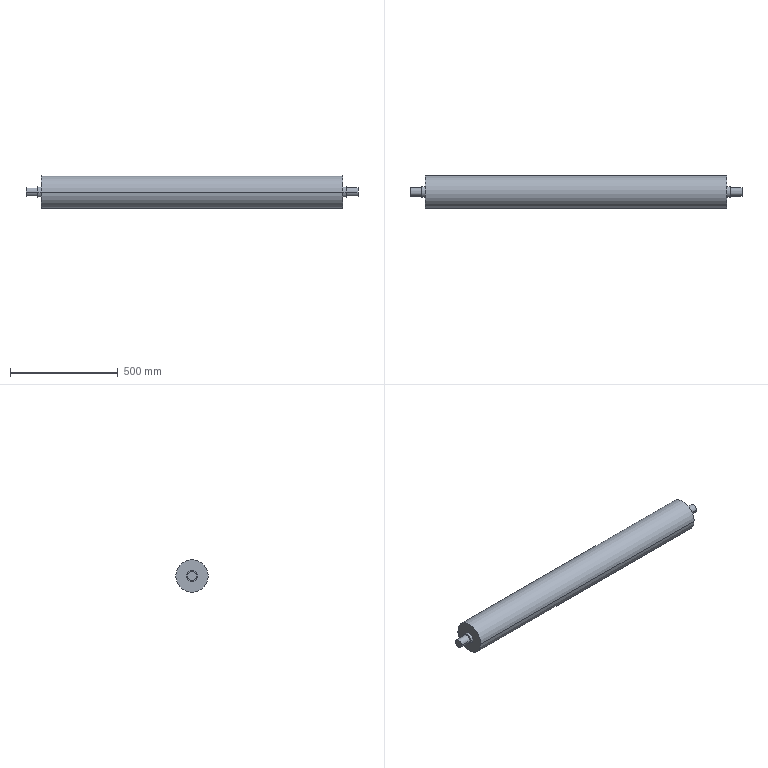Part | SolidWorks | features BaseBody 1 | 1 solid | 16 faces | box 1540 x 150 x 150 mm | volume 24937177 mm3 | cylinder 10 | plane 6 | commonest cylinder face diameters 40 x4 50 x4 150 x2
STEP:
#1=CARTESIAN_POINT('',(-715.,-20.,0.));
#2=VERTEX_POINT('',#1);
#3=CARTESIAN_POINT('',(-715.,20.,0.));
#4=VERTEX_POINT('',#3);
#5=CARTESIAN_POINT('',(-715.,0.,0.));
#6=DIRECTION('',(-1.,0.,0.));
#7=DIRECTION('',(0.,1.,0.));
#8=AXIS2_PLACEMENT_3D('',#5,#6,#7);
#9=CIRCLE('',#8,20.);
#10=EDGE_CURVE('',#2,#4,#9,.T.);
#11=ORIENTED_EDGE('',*,*,#10,.T.);
#12=CARTESIAN_POINT('',(-770.,20.,0.));
#13=VERTEX_POINT('',#12);
#14=CARTESIAN_POINT('',(-820.,20.,0.));
#15=DIRECTION('',(-1.,0.,0.));
#16=VECTOR('',#15,1000.);
#17=LINE('',#14,#16);
#18=EDGE_CURVE('',#4,#13,#17,.T.);
#19=ORIENTED_EDGE('',*,*,#18,.T.);
#20=CARTESIAN_POINT('',(-770.,-20.,0.));
#21=VERTEX_POINT('',#20);
#22=CARTESIAN_POINT('',(-770.,0.,0.));
#23=DIRECTION('',(-1.,0.,0.));
#24=DIRECTION('',(0.,-1.,0.));
#25=AXIS2_PLACEMENT_3D('',#22,#23,#24);
#26=CIRCLE('',#25,20.);
#27=EDGE_CURVE('',#21,#13,#26,.T.);
#28=ORIENTED_EDGE('',*,*,#27,.F.);
#29=CARTESIAN_POINT('',(-820.,-20.,0.));
#30=DIRECTION('',(-1.,0.,0.));
#31=VECTOR('',#30,1000.);
#32=LINE('',#29,#31);
#33=EDGE_CURVE('',#2,#21,#32,.T.);
#34=ORIENTED_EDGE('',*,*,#33,.F.);
#35=EDGE_LOOP('',(#11,#19,#28,#34));
#36=FACE_OUTER_BOUND('',#35,.T.);
#37=CARTESIAN_POINT('',(-820.,0.,0.));
#38=DIRECTION('',(-1.,0.,0.));
#39=DIRECTION('',(0.,-1.,0.));
#40=AXIS2_PLACEMENT_3D('',#37,#38,#39);
#41=CYLINDRICAL_SURFACE('',#40,20.);
#42=ADVANCED_FACE('',(#36),#41,.T.);
#43=CARTESIAN_POINT('',(-700.,-25.,0.));
#44=VERTEX_POINT('',#43);
#45=CARTESIAN_POINT('',(-700.,25.,0.));
#46=VERTEX_POINT('',#45);
#47=CARTESIAN_POINT('',(-700.,0.,0.));
#48=DIRECTION('',(-1.,0.,0.));
#49=DIRECTION('',(0.,1.,0.));
#50=AXIS2_PLACEMENT_3D('',#47,#48,#49);
#51=CIRCLE('',#50,25.);
#52=EDGE_CURVE('',#44,#46,#51,.T.);
#53=ORIENTED_EDGE('',*,*,#52,.T.);
#54=CARTESIAN_POINT('',(-715.,25.,0.));
#55=VERTEX_POINT('',#54);
#56=CARTESIAN_POINT('',(-820.,25.,0.));
#57=DIRECTION('',(-1.,0.,0.));
#58=VECTOR('',#57,1000.);
#59=LINE('',#56,#58);
#60=EDGE_CURVE('',#46,#55,#59,.T.);
#61=ORIENTED_EDGE('',*,*,#60,.T.);
#62=CARTESIAN_POINT('',(-715.,-25.,0.));
#63=VERTEX_POINT('',#62);
#64=CARTESIAN_POINT('',(-715.,0.,0.));
#65=DIRECTION('',(-1.,0.,0.));
#66=DIRECTION('',(0.,-1.,0.));
#67=AXIS2_PLACEMENT_3D('',#64,#65,#66);
#68=CIRCLE('',#67,25.);
#69=EDGE_CURVE('',#63,#55,#68,.T.);
#70=ORIENTED_EDGE('',*,*,#69,.F.);
#71=CARTESIAN_POINT('',(-820.,-25.,0.));
#72=DIRECTION('',(-1.,0.,0.));
#73=VECTOR('',#72,1000.);
#74=LINE('',#71,#73);
#75=EDGE_CURVE('',#44,#63,#74,.T.);
#76=ORIENTED_EDGE('',*,*,#75,.F.);
#77=EDGE_LOOP('',(#53,#61,#70,#76));
#78=FACE_OUTER_BOUND('',#77,.T.);
#79=CARTESIAN_POINT('',(-820.,0.,0.));
#80=DIRECTION('',(-1.,0.,0.));
#81=DIRECTION('',(0.,-1.,0.));
#82=AXIS2_PLACEMENT_3D('',#79,#80,#81);
#83=CYLINDRICAL_SURFACE('',#82,25.);
#84=ADVANCED_FACE('',(#78),#83,.T.);
#85=CARTESIAN_POINT('',(770.,-20.,0.));
#86=VERTEX_POINT('',#85);
#87=CARTESIAN_POINT('',(770.,20.,0.));
#88=VERTEX_POINT('',#87);
#89=CARTESIAN_POINT('',(770.,0.,0.));
#90=DIRECTION('',(-1.,0.,0.));
#91=DIRECTION('',(0.,-1.,0.));
#92=AXIS2_PLACEMENT_3D('',#89,#90,#91);
#93=CIRCLE('',#92,20.);
#94=EDGE_CURVE('',#86,#88,#93,.T.);
#95=ORIENTED_EDGE('',*,*,#94,.T.);
#96=CARTESIAN_POINT('',(715.,20.,0.));
#97=VERTEX_POINT('',#96);
#98=CARTESIAN_POINT('',(-820.,20.,0.));
#99=DIRECTION('',(-1.,0.,0.));
#100=VECTOR('',#99,1000.);
#101=LINE('',#98,#100);
#102=EDGE_CURVE('',#88,#97,#101,.T.);
#103=ORIENTED_EDGE('',*,*,#102,.T.);
#104=CARTESIAN_POINT('',(715.,-20.,0.));
#105=VERTEX_POINT('',#104);
#106=CARTESIAN_POINT('',(715.,0.,0.));
#107=DIRECTION('',(1.,0.,0.));
#108=DIRECTION('',(0.,-1.,0.));
#109=AXIS2_PLACEMENT_3D('',#106,#107,#108);
#110=CIRCLE('',#109,20.);
#111=EDGE_CURVE('',#97,#105,#110,.T.);
#112=ORIENTED_EDGE('',*,*,#111,.T.);
#113=CARTESIAN_POINT('',(-820.,-20.,0.));
#114=DIRECTION('',(-1.,0.,0.));
#115=VECTOR('',#114,1000.);
#116=LINE('',#113,#115);
#117=EDGE_CURVE('',#86,#105,#116,.T.);
#118=ORIENTED_EDGE('',*,*,#117,.F.);
#119=EDGE_LOOP('',(#95,#103,#112,#118));
#120=FACE_OUTER_BOUND('',#119,.T.);
#121=CARTESIAN_POINT('',(-820.,0.,0.));
#122=DIRECTION('',(-1.,0.,0.));
#123=DIRECTION('',(0.,-1.,0.));
#124=AXIS2_PLACEMENT_3D('',#121,#122,#123);
#125=CYLINDRICAL_SURFACE('',#124,20.);
#126=ADVANCED_FACE('',(#120),#125,.T.);
#127=CARTESIAN_POINT('',(715.,-25.,0.));
#128=VERTEX_POINT('',#127);
#129=CARTESIAN_POINT('',(715.,25.,0.));
#130=VERTEX_POINT('',#129);
#131=CARTESIAN_POINT('',(715.,0.,0.));
#132=DIRECTION('',(-1.,0.,0.));
#133=DIRECTION('',(0.,-1.,0.));
#134=AXIS2_PLACEMENT_3D('',#131,#132,#133);
#135=CIRCLE('',#134,25.);
#136=EDGE_CURVE('',#128,#130,#135,.T.);
#137=ORIENTED_EDGE('',*,*,#136,.T.);
#138=CARTESIAN_POINT('',(700.,25.,0.));
#139=VERTEX_POINT('',#138);
#140=CARTESIAN_POINT('',(-820.,25.,0.));
#141=DIRECTION('',(-1.,0.,0.));
#142=VECTOR('',#141,1000.);
#143=LINE('',#140,#142);
#144=EDGE_CURVE('',#130,#139,#143,.T.);
#145=ORIENTED_EDGE('',*,*,#144,.T.);
#146=CARTESIAN_POINT('',(700.,-25.,0.));
#147=VERTEX_POINT('',#146);
#148=CARTESIAN_POINT('',(700.,0.,0.));
#149=DIRECTION('',(1.,0.,0.));
#150=DIRECTION('',(0.,-1.,0.));
#151=AXIS2_PLACEMENT_3D('',#148,#149,#150);
#152=CIRCLE('',#151,25.);
#153=EDGE_CURVE('',#139,#147,#152,.T.);
#154=ORIENTED_EDGE('',*,*,#153,.T.);
#155=CARTESIAN_POINT('',(-820.,-25.,0.));
#156=DIRECTION('',(-1.,0.,0.));
#157=VECTOR('',#156,1000.);
#158=LINE('',#155,#157);
#159=EDGE_CURVE('',#128,#147,#158,.T.);
#160=ORIENTED_EDGE('',*,*,#159,.F.);
#161=EDGE_LOOP('',(#137,#145,#154,#160));
#162=FACE_OUTER_BOUND('',#161,.T.);
#163=CARTESIAN_POINT('',(-820.,0.,0.));
#164=DIRECTION('',(-1.,0.,0.));
#165=DIRECTION('',(0.,-1.,0.));
#166=AXIS2_PLACEMENT_3D('',#163,#164,#165);
#167=CYLINDRICAL_SURFACE('',#166,25.);
#168=ADVANCED_FACE('',(#162),#167,.T.);
#169=CARTESIAN_POINT('',(700.,-75.,0.));
#170=VERTEX_POINT('',#169);
#171=CARTESIAN_POINT('',(700.,75.,0.));
#172=VERTEX_POINT('',#171);
#173=CARTESIAN_POINT('',(700.,0.,0.));
#174=DIRECTION('',(-1.,0.,0.));
#175=DIRECTION('',(0.,-1.,0.));
#176=AXIS2_PLACEMENT_3D('',#173,#174,#175);
#177=CIRCLE('',#176,75.);
#178=EDGE_CURVE('',#170,#172,#177,.T.);
#179=ORIENTED_EDGE('',*,*,#178,.T.);
#180=CARTESIAN_POINT('',(-700.,75.,0.));
#181=VERTEX_POINT('',#180);
#182=CARTESIAN_POINT('',(-820.,75.,0.));
#183=DIRECTION('',(-1.,0.,0.));
#184=VECTOR('',#183,1000.);
#185=LINE('',#182,#184);
#186=EDGE_CURVE('',#172,#181,#185,.T.);
#187=ORIENTED_EDGE('',*,*,#186,.T.);
#188=CARTESIAN_POINT('',(-700.,-75.,0.));
#189=VERTEX_POINT('',#188);
#190=CARTESIAN_POINT('',(-700.,0.,0.));
#191=DIRECTION('',(-1.,0.,0.));
#192=DIRECTION('',(0.,-1.,0.));
#193=AXIS2_PLACEMENT_3D('',#190,#191,#192);
#194=CIRCLE('',#193,75.);
#195=EDGE_CURVE('',#189,#181,#194,.T.);
#196=ORIENTED_EDGE('',*,*,#195,.F.);
#197=CARTESIAN_POINT('',(-820.,-75.,0.));
#198=DIRECTION('',(-1.,0.,0.));
#199=VECTOR('',#198,1000.);
#200=LINE('',#197,#199);
#201=EDGE_CURVE('',#170,#189,#200,.T.);
#202=ORIENTED_EDGE('',*,*,#201,.F.);
#203=EDGE_LOOP('',(#179,#187,#196,#202));
#204=FACE_OUTER_BOUND('',#203,.T.);
#205=CARTESIAN_POINT('',(-820.,0.,0.));
#206=DIRECTION('',(-1.,0.,0.));
#207=DIRECTION('',(0.,-1.,0.));
#208=AXIS2_PLACEMENT_3D('',#205,#206,#207);
#209=CYLINDRICAL_SURFACE('',#208,75.);
#210=ADVANCED_FACE('',(#204),#209,.T.);
#211=ORIENTED_EDGE('',*,*,#27,.T.);
#212=CARTESIAN_POINT('',(-770.,0.,0.));
#213=DIRECTION('',(-1.,0.,0.));
#214=DIRECTION('',(0.,-1.,0.));
#215=AXIS2_PLACEMENT_3D('',#212,#213,#214);
#216=CIRCLE('',#215,20.);
#217=EDGE_CURVE('',#13,#21,#216,.T.);
#218=ORIENTED_EDGE('',*,*,#217,.T.);
#219=EDGE_LOOP('',(#211,#218));
#220=FACE_OUTER_BOUND('',#219,.T.);
#221=CARTESIAN_POINT('',(-770.,17.5,0.));
#222=DIRECTION('',(1.,0.,0.));
#223=DIRECTION('',(0.,-1.,0.));
#224=AXIS2_PLACEMENT_3D('',#221,#222,#223);
#225=PLANE('',#224);
#226=ADVANCED_FACE('',(#220),#225,.F.);
#227=ORIENTED_EDGE('',*,*,#10,.F.);
#228=CARTESIAN_POINT('',(-715.,0.,0.));
#229=DIRECTION('',(-1.,0.,0.));
#230=DIRECTION('',(0.,1.,0.));
#231=AXIS2_PLACEMENT_3D('',#228,#229,#230);
#232=CIRCLE('',#231,20.);
#233=EDGE_CURVE('',#4,#2,#232,.T.);
#234=ORIENTED_EDGE('',*,*,#233,.F.);
#235=EDGE_LOOP('',(#227,#234));
#236=FACE_BOUND('',#235,.T.);
#237=ORIENTED_EDGE('',*,*,#69,.T.);
#238=CARTESIAN_POINT('',(-715.,0.,0.));
#239=DIRECTION('',(-1.,0.,0.));
#240=DIRECTION('',(0.,-1.,0.));
#241=AXIS2_PLACEMENT_3D('',#238,#239,#240);
#242=CIRCLE('',#241,25.);
#243=EDGE_CURVE('',#55,#63,#242,.T.);
#244=ORIENTED_EDGE('',*,*,#243,.T.);
#245=EDGE_LOOP('',(#237,#244));
#246=FACE_OUTER_BOUND('',#245,.T.);
#247=CARTESIAN_POINT('',(-715.,20.,0.));
#248=DIRECTION('',(1.,0.,0.));
#249=DIRECTION('',(0.,-1.,0.));
#250=AXIS2_PLACEMENT_3D('',#247,#248,#249);
#251=PLANE('',#250);
#252=ADVANCED_FACE('',(#236,#246),#251,.F.);
#253=ORIENTED_EDGE('',*,*,#94,.F.);
#254=CARTESIAN_POINT('',(770.,0.,0.));
#255=DIRECTION('',(-1.,0.,0.));
#256=DIRECTION('',(0.,-1.,0.));
#257=AXIS2_PLACEMENT_3D('',#254,#255,#256);
#258=CIRCLE('',#257,20.);
#259=EDGE_CURVE('',#88,#86,#258,.T.);
#260=ORIENTED_EDGE('',*,*,#259,.F.);
#261=EDGE_LOOP('',(#253,#260));
#262=FACE_OUTER_BOUND('',#261,.T.);
#263=CARTESIAN_POINT('',(770.,17.5,0.));
#264=DIRECTION('',(-1.,0.,0.));
#265=DIRECTION('',(0.,0.,1.));
#266=AXIS2_PLACEMENT_3D('',#263,#264,#265);
#267=PLANE('',#266);
#268=ADVANCED_FACE('',(#262),#267,.F.);
#269=CARTESIAN_POINT('',(715.,0.,0.));
#270=DIRECTION('',(1.,0.,0.));
#271=DIRECTION('',(0.,-1.,0.));
#272=AXIS2_PLACEMENT_3D('',#269,#270,#271);
#273=CIRCLE('',#272,20.);
#274=EDGE_CURVE('',#105,#97,#273,.T.);
#275=ORIENTED_EDGE('',*,*,#274,.F.);
#276=ORIENTED_EDGE('',*,*,#111,.F.);
#277=EDGE_LOOP('',(#275,#276));
#278=FACE_BOUND('',#277,.T.);
#279=ORIENTED_EDGE('',*,*,#136,.F.);
#280=CARTESIAN_POINT('',(715.,0.,0.));
#281=DIRECTION('',(-1.,0.,0.));
#282=DIRECTION('',(0.,-1.,0.));
#283=AXIS2_PLACEMENT_3D('',#280,#281,#282);
#284=CIRCLE('',#283,25.);
#285=EDGE_CURVE('',#130,#128,#284,.T.);
#286=ORIENTED_EDGE('',*,*,#285,.F.);
#287=EDGE_LOOP('',(#279,#286));
#288=FACE_OUTER_BOUND('',#287,.T.);
#289=CARTESIAN_POINT('',(715.,20.,0.));
#290=DIRECTION('',(-1.,0.,0.));
#291=DIRECTION('',(0.,0.,1.));
#292=AXIS2_PLACEMENT_3D('',#289,#290,#291);
#293=PLANE('',#292);
#294=ADVANCED_FACE('',(#278,#288),#293,.F.);
#295=CARTESIAN_POINT('',(700.,0.,0.));
#296=DIRECTION('',(1.,0.,0.));
#297=DIRECTION('',(0.,-1.,0.));
#298=AXIS2_PLACEMENT_3D('',#295,#296,#297);
#299=CIRCLE('',#298,25.);
#300=EDGE_CURVE('',#147,#139,#299,.T.);
#301=ORIENTED_EDGE('',*,*,#300,.F.);
#302=ORIENTED_EDGE('',*,*,#153,.F.);
#303=EDGE_LOOP('',(#301,#302));
#304=FACE_BOUND('',#303,.T.);
#305=ORIENTED_EDGE('',*,*,#178,.F.);
#306=CARTESIAN_POINT('',(700.,0.,0.));
#307=DIRECTION('',(-1.,0.,0.));
#308=DIRECTION('',(0.,-1.,0.));
#309=AXIS2_PLACEMENT_3D('',#306,#307,#308);
#310=CIRCLE('',#309,75.);
#311=EDGE_CURVE('',#172,#170,#310,.T.);
#312=ORIENTED_EDGE('',*,*,#311,.F.);
#313=EDGE_LOOP('',(#305,#312));
#314=FACE_OUTER_BOUND('',#313,.T.);
#315=CARTESIAN_POINT('',(700.,75.,0.));
#316=DIRECTION('',(-1.,0.,0.));
#317=DIRECTION('',(0.,0.,1.));
#318=AXIS2_PLACEMENT_3D('',#315,#316,#317);
#319=PLANE('',#318);
#320=ADVANCED_FACE('',(#304,#314),#319,.F.);
#321=ORIENTED_EDGE('',*,*,#52,.F.);
#322=CARTESIAN_POINT('',(-700.,0.,0.));
#323=DIRECTION('',(-1.,0.,0.));
#324=DIRECTION('',(0.,1.,0.));
#325=AXIS2_PLACEMENT_3D('',#322,#323,#324);
#326=CIRCLE('',#325,25.);
#327=EDGE_CURVE('',#46,#44,#326,.T.);
#328=ORIENTED_EDGE('',*,*,#327,.F.);
#329=EDGE_LOOP('',(#321,#328));
#330=FACE_BOUND('',#329,.T.);
#331=ORIENTED_EDGE('',*,*,#195,.T.);
#332=CARTESIAN_POINT('',(-700.,0.,0.));
#333=DIRECTION('',(-1.,0.,0.));
#334=DIRECTION('',(0.,-1.,0.));
#335=AXIS2_PLACEMENT_3D('',#332,#333,#334);
#336=CIRCLE('',#335,75.);
#337=EDGE_CURVE('',#181,#189,#336,.T.);
#338=ORIENTED_EDGE('',*,*,#337,.T.);
#339=EDGE_LOOP('',(#331,#338));
#340=FACE_OUTER_BOUND('',#339,.T.);
#341=CARTESIAN_POINT('',(-700.,75.,0.));
#342=DIRECTION('',(1.,0.,0.));
#343=DIRECTION('',(0.,-1.,0.));
#344=AXIS2_PLACEMENT_3D('',#341,#342,#343);
#345=PLANE('',#344);
#346=ADVANCED_FACE('',(#330,#340),#345,.F.);
#347=ORIENTED_EDGE('',*,*,#186,.F.);
#348=ORIENTED_EDGE('',*,*,#311,.T.);
#349=ORIENTED_EDGE('',*,*,#201,.T.);
#350=ORIENTED_EDGE('',*,*,#337,.F.);
#351=EDGE_LOOP('',(#347,#348,#349,#350));
#352=FACE_OUTER_BOUND('',#351,.T.);
#353=CARTESIAN_POINT('',(-820.,0.,0.));
#354=DIRECTION('',(-1.,0.,0.));
#355=DIRECTION('',(0.,-1.,0.));
#356=AXIS2_PLACEMENT_3D('',#353,#354,#355);
#357=CYLINDRICAL_SURFACE('',#356,75.);
#358=ADVANCED_FACE('',(#352),#357,.T.);
#359=ORIENTED_EDGE('',*,*,#144,.F.);
#360=ORIENTED_EDGE('',*,*,#285,.T.);
#361=ORIENTED_EDGE('',*,*,#159,.T.);
#362=ORIENTED_EDGE('',*,*,#300,.T.);
#363=EDGE_LOOP('',(#359,#360,#361,#362));
#364=FACE_OUTER_BOUND('',#363,.T.);
#365=CARTESIAN_POINT('',(-820.,0.,0.));
#366=DIRECTION('',(-1.,0.,0.));
#367=DIRECTION('',(0.,-1.,0.));
#368=AXIS2_PLACEMENT_3D('',#365,#366,#367);
#369=CYLINDRICAL_SURFACE('',#368,25.);
#370=ADVANCED_FACE('',(#364),#369,.T.);
#371=ORIENTED_EDGE('',*,*,#102,.F.);
#372=ORIENTED_EDGE('',*,*,#259,.T.);
#373=ORIENTED_EDGE('',*,*,#117,.T.);
#374=ORIENTED_EDGE('',*,*,#274,.T.);
#375=EDGE_LOOP('',(#371,#372,#373,#374));
#376=FACE_OUTER_BOUND('',#375,.T.);
#377=CARTESIAN_POINT('',(-820.,0.,0.));
#378=DIRECTION('',(-1.,0.,0.));
#379=DIRECTION('',(0.,-1.,0.));
#380=AXIS2_PLACEMENT_3D('',#377,#378,#379);
#381=CYLINDRICAL_SURFACE('',#380,20.);
#382=ADVANCED_FACE('',(#376),#381,.T.);
#383=ORIENTED_EDGE('',*,*,#60,.F.);
#384=ORIENTED_EDGE('',*,*,#327,.T.);
#385=ORIENTED_EDGE('',*,*,#75,.T.);
#386=ORIENTED_EDGE('',*,*,#243,.F.);
#387=EDGE_LOOP('',(#383,#384,#385,#386));
#388=FACE_OUTER_BOUND('',#387,.T.);
#389=CARTESIAN_POINT('',(-820.,0.,0.));
#390=DIRECTION('',(-1.,0.,0.));
#391=DIRECTION('',(0.,-1.,0.));
#392=AXIS2_PLACEMENT_3D('',#389,#390,#391);
#393=CYLINDRICAL_SURFACE('',#392,25.);
#394=ADVANCED_FACE('',(#388),#393,.T.);
#395=ORIENTED_EDGE('',*,*,#18,.F.);
#396=ORIENTED_EDGE('',*,*,#233,.T.);
#397=ORIENTED_EDGE('',*,*,#33,.T.);
#398=ORIENTED_EDGE('',*,*,#217,.F.);
#399=EDGE_LOOP('',(#395,#396,#397,#398));
#400=FACE_OUTER_BOUND('',#399,.T.);
#401=CARTESIAN_POINT('',(-820.,0.,0.));
#402=DIRECTION('',(-1.,0.,0.));
#403=DIRECTION('',(0.,-1.,0.));
#404=AXIS2_PLACEMENT_3D('',#401,#402,#403);
#405=CYLINDRICAL_SURFACE('',#404,20.);
#406=ADVANCED_FACE('',(#400),#405,.T.);
#407=CLOSED_SHELL('',(#42,#84,#126,#168,#210,#226,#252,#268,#294,#320,#346,#358,#370,#382,#394,#406));
#408=MANIFOLD_SOLID_BREP('',#407);
#409=CARTESIAN_POINT('',(0.,0.,0.));
#410=DIRECTION('',(0.,0.,1.));
#411=DIRECTION('',(1.,0.,0.));
#412=AXIS2_PLACEMENT_3D('',#409,#410,#411);
#413=(LENGTH_UNIT()NAMED_UNIT(*)SI_UNIT(.MILLI.,.METRE.));
#414=UNCERTAINTY_MEASURE_WITH_UNIT(LENGTH_MEASURE(0.00001),#413,'','');
#415=(NAMED_UNIT(*)PLANE_ANGLE_UNIT()SI_UNIT($,.RADIAN.));
#416=(NAMED_UNIT(*)SI_UNIT($,.STERADIAN.)SOLID_ANGLE_UNIT());
#417=(GEOMETRIC_REPRESENTATION_CONTEXT(3)GLOBAL_UNCERTAINTY_ASSIGNED_CONTEXT((#414))GLOBAL_UNIT_ASSIGNED_CONTEXT((#413,#415,#416))REPRESENTATION_CONTEXT('',''));
#418=ADVANCED_BREP_SHAPE_REPRESENTATION('',(#408,#412),#417);